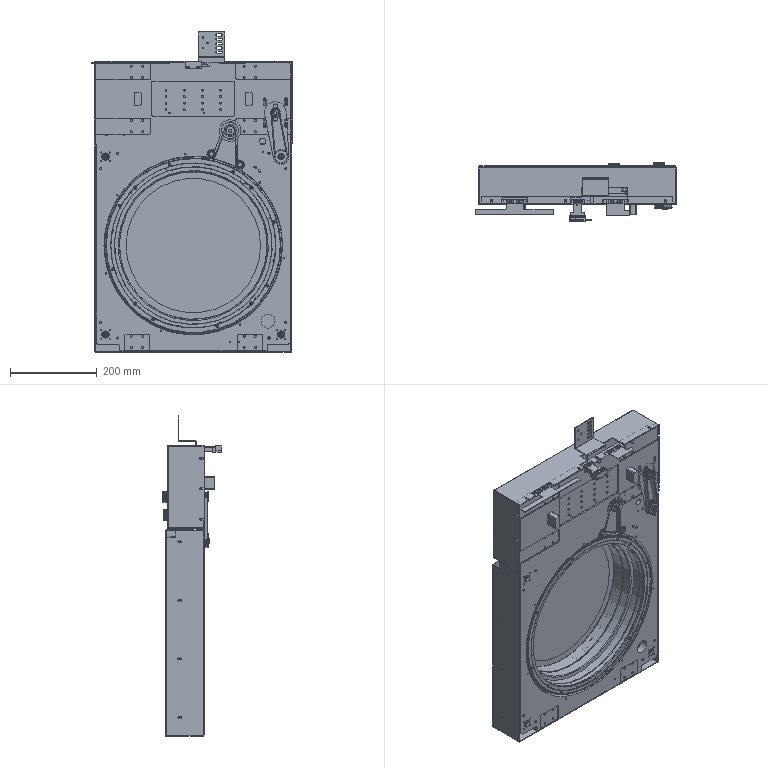Part | NX | features BREP 68 | 240 solids | 16117 faces | volume 6738834 mm3 | cylinder 8622 | plane 4492 | cone 1606 | torus 665 | sphere 596 | spline 136 | commonest cylinder face diameters 3.04 x1048 0.5 x1022 25 x742 1.7 x649 10 x459 4 x448